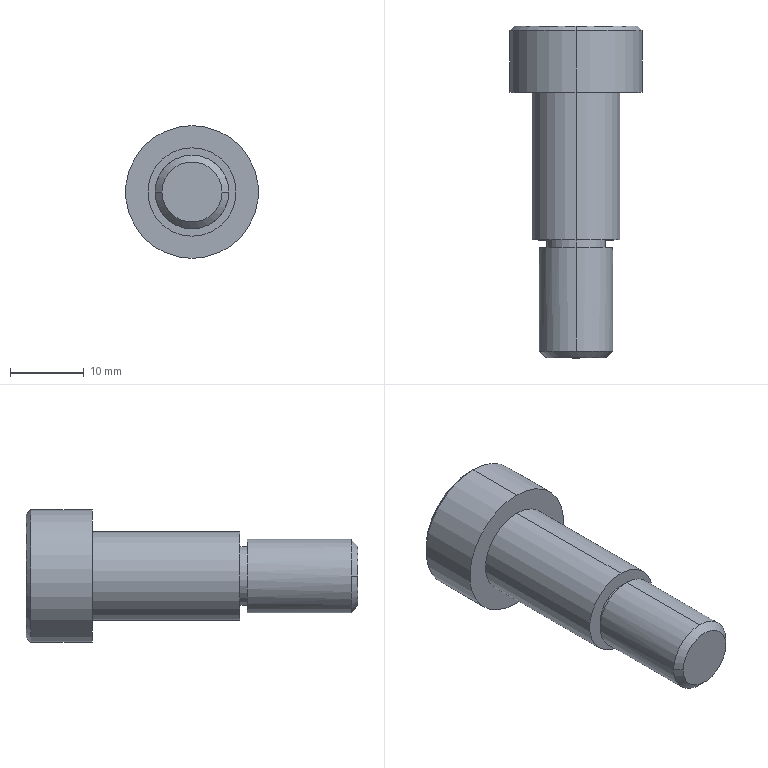Part | SolidWorks | features BaseBody 1, MoveFace 1 | 1 solid | 24 faces | box 18 x 45 x 18 mm | volume 5618 mm3 | plane 12 | cylinder 8 | cone 4 | commonest cylinder face diameters 8 x2 10 x2 12 x2 18 x2
STEP:
#1=CARTESIAN_POINT('',(0.,12.,6.));
#2=VERTEX_POINT('',#1);
#3=CARTESIAN_POINT('',(0.,12.,-6.));
#4=VERTEX_POINT('',#3);
#5=CARTESIAN_POINT('',(0.,12.,0.));
#6=DIRECTION('',(0.,1.,0.));
#7=DIRECTION('',(0.,0.,1.));
#8=AXIS2_PLACEMENT_3D('',#5,#6,#7);
#9=CIRCLE('',#8,6.);
#10=EDGE_CURVE('',#2,#4,#9,.T.);
#11=ORIENTED_EDGE('',*,*,#10,.T.);
#12=CARTESIAN_POINT('',(0.,32.,-6.));
#13=VERTEX_POINT('',#12);
#14=CARTESIAN_POINT('',(0.,0.,-6.));
#15=DIRECTION('',(0.,1.,0.));
#16=VECTOR('',#15,1000.);
#17=LINE('',#14,#16);
#18=EDGE_CURVE('',#4,#13,#17,.T.);
#19=ORIENTED_EDGE('',*,*,#18,.T.);
#20=CARTESIAN_POINT('',(0.,32.,6.));
#21=VERTEX_POINT('',#20);
#22=CARTESIAN_POINT('',(0.,32.,0.));
#23=DIRECTION('',(0.,-1.,0.));
#24=DIRECTION('',(0.,0.,1.));
#25=AXIS2_PLACEMENT_3D('',#22,#23,#24);
#26=CIRCLE('',#25,6.);
#27=EDGE_CURVE('',#13,#21,#26,.T.);
#28=ORIENTED_EDGE('',*,*,#27,.T.);
#29=CARTESIAN_POINT('',(0.,0.,6.));
#30=DIRECTION('',(0.,1.,0.));
#31=VECTOR('',#30,1000.);
#32=LINE('',#29,#31);
#33=EDGE_CURVE('',#2,#21,#32,.T.);
#34=ORIENTED_EDGE('',*,*,#33,.F.);
#35=EDGE_LOOP('',(#11,#19,#28,#34));
#36=FACE_OUTER_BOUND('',#35,.T.);
#37=CARTESIAN_POINT('',(0.,0.,0.));
#38=DIRECTION('',(0.,1.,0.));
#39=DIRECTION('',(0.,0.,1.));
#40=AXIS2_PLACEMENT_3D('',#37,#38,#39);
#41=CYLINDRICAL_SURFACE('',#40,6.);
#42=ADVANCED_FACE('',(#36),#41,.T.);
#43=CARTESIAN_POINT('',(0.,32.,9.));
#44=VERTEX_POINT('',#43);
#45=CARTESIAN_POINT('',(0.,32.,-9.));
#46=VERTEX_POINT('',#45);
#47=CARTESIAN_POINT('',(0.,32.,0.));
#48=DIRECTION('',(0.,1.,0.));
#49=DIRECTION('',(0.,0.,1.));
#50=AXIS2_PLACEMENT_3D('',#47,#48,#49);
#51=CIRCLE('',#50,9.);
#52=EDGE_CURVE('',#44,#46,#51,.T.);
#53=ORIENTED_EDGE('',*,*,#52,.T.);
#54=CARTESIAN_POINT('',(0.,40.4,-9.));
#55=VERTEX_POINT('',#54);
#56=CARTESIAN_POINT('',(0.,0.,-9.));
#57=DIRECTION('',(0.,1.,0.));
#58=VECTOR('',#57,1000.);
#59=LINE('',#56,#58);
#60=EDGE_CURVE('',#46,#55,#59,.T.);
#61=ORIENTED_EDGE('',*,*,#60,.T.);
#62=CARTESIAN_POINT('',(0.,40.4,9.));
#63=VERTEX_POINT('',#62);
#64=CARTESIAN_POINT('',(0.,40.4,0.));
#65=DIRECTION('',(0.,-1.,0.));
#66=DIRECTION('',(0.,0.,1.));
#67=AXIS2_PLACEMENT_3D('',#64,#65,#66);
#68=CIRCLE('',#67,9.);
#69=EDGE_CURVE('',#55,#63,#68,.T.);
#70=ORIENTED_EDGE('',*,*,#69,.T.);
#71=CARTESIAN_POINT('',(0.,0.,9.));
#72=DIRECTION('',(0.,1.,0.));
#73=VECTOR('',#72,1000.);
#74=LINE('',#71,#73);
#75=EDGE_CURVE('',#44,#63,#74,.T.);
#76=ORIENTED_EDGE('',*,*,#75,.F.);
#77=EDGE_LOOP('',(#53,#61,#70,#76));
#78=FACE_OUTER_BOUND('',#77,.T.);
#79=CARTESIAN_POINT('',(0.,0.,0.));
#80=DIRECTION('',(0.,1.,0.));
#81=DIRECTION('',(0.,0.,1.));
#82=AXIS2_PLACEMENT_3D('',#79,#80,#81);
#83=CYLINDRICAL_SURFACE('',#82,9.);
#84=ADVANCED_FACE('',(#78),#83,.T.);
#85=CARTESIAN_POINT('',(0.,11.,4.));
#86=VERTEX_POINT('',#85);
#87=CARTESIAN_POINT('',(0.,11.,-4.));
#88=VERTEX_POINT('',#87);
#89=CARTESIAN_POINT('',(0.,11.,0.));
#90=DIRECTION('',(0.,1.,0.));
#91=DIRECTION('',(0.,0.,1.));
#92=AXIS2_PLACEMENT_3D('',#89,#90,#91);
#93=CIRCLE('',#92,4.);
#94=EDGE_CURVE('',#86,#88,#93,.T.);
#95=ORIENTED_EDGE('',*,*,#94,.T.);
#96=CARTESIAN_POINT('',(0.,12.,-4.));
#97=VERTEX_POINT('',#96);
#98=CARTESIAN_POINT('',(0.,0.,-4.));
#99=DIRECTION('',(0.,1.,0.));
#100=VECTOR('',#99,1000.);
#101=LINE('',#98,#100);
#102=EDGE_CURVE('',#88,#97,#101,.T.);
#103=ORIENTED_EDGE('',*,*,#102,.T.);
#104=CARTESIAN_POINT('',(0.,12.,4.));
#105=VERTEX_POINT('',#104);
#106=CARTESIAN_POINT('',(0.,12.,0.));
#107=DIRECTION('',(0.,-1.,0.));
#108=DIRECTION('',(0.,0.,1.));
#109=AXIS2_PLACEMENT_3D('',#106,#107,#108);
#110=CIRCLE('',#109,4.);
#111=EDGE_CURVE('',#97,#105,#110,.T.);
#112=ORIENTED_EDGE('',*,*,#111,.T.);
#113=CARTESIAN_POINT('',(0.,0.,4.));
#114=DIRECTION('',(0.,1.,0.));
#115=VECTOR('',#114,1000.);
#116=LINE('',#113,#115);
#117=EDGE_CURVE('',#86,#105,#116,.T.);
#118=ORIENTED_EDGE('',*,*,#117,.F.);
#119=EDGE_LOOP('',(#95,#103,#112,#118));
#120=FACE_OUTER_BOUND('',#119,.T.);
#121=CARTESIAN_POINT('',(0.,0.,0.));
#122=DIRECTION('',(0.,1.,0.));
#123=DIRECTION('',(0.,0.,1.));
#124=AXIS2_PLACEMENT_3D('',#121,#122,#123);
#125=CYLINDRICAL_SURFACE('',#124,4.);
#126=ADVANCED_FACE('',(#120),#125,.T.);
#127=CARTESIAN_POINT('',(0.,41.,-8.4));
#128=VERTEX_POINT('',#127);
#129=CARTESIAN_POINT('',(0.,41.,8.4));
#130=VERTEX_POINT('',#129);
#131=CARTESIAN_POINT('',(0.,41.,0.));
#132=DIRECTION('',(0.,-1.,0.));
#133=DIRECTION('',(0.,0.,-1.));
#134=AXIS2_PLACEMENT_3D('',#131,#132,#133);
#135=CIRCLE('',#134,8.4);
#136=EDGE_CURVE('',#128,#130,#135,.T.);
#137=ORIENTED_EDGE('',*,*,#136,.T.);
#138=CARTESIAN_POINT('',(0.,40.4,9.));
#139=DIRECTION('',(0.,-0.7071,0.7071));
#140=VECTOR('',#139,1000.);
#141=LINE('',#138,#140);
#142=EDGE_CURVE('',#130,#63,#141,.T.);
#143=ORIENTED_EDGE('',*,*,#142,.T.);
#144=ORIENTED_EDGE('',*,*,#69,.F.);
#145=CARTESIAN_POINT('',(0.,40.4,-9.));
#146=DIRECTION('',(0.,-0.7071,-0.7071));
#147=VECTOR('',#146,1000.);
#148=LINE('',#145,#147);
#149=EDGE_CURVE('',#128,#55,#148,.T.);
#150=ORIENTED_EDGE('',*,*,#149,.F.);
#151=EDGE_LOOP('',(#137,#143,#144,#150));
#152=FACE_OUTER_BOUND('',#151,.T.);
#153=CARTESIAN_POINT('',(0.,40.4,0.));
#154=DIRECTION('',(0.,-1.,0.));
#155=DIRECTION('',(0.,0.,-1.));
#156=AXIS2_PLACEMENT_3D('',#153,#154,#155);
#157=CONICAL_SURFACE('',#156,9.,0.7854);
#158=ADVANCED_FACE('',(#152),#157,.T.);
#159=CARTESIAN_POINT('',(5.,-3.08,0.));
#160=VERTEX_POINT('',#159);
#161=CARTESIAN_POINT('',(0.,-3.08,-5.));
#162=VERTEX_POINT('',#161);
#163=CARTESIAN_POINT('',(0.,-3.08,0.));
#164=DIRECTION('',(0.,1.,0.));
#165=DIRECTION('',(0.,0.,1.));
#166=AXIS2_PLACEMENT_3D('',#163,#164,#165);
#167=CIRCLE('',#166,5.);
#168=EDGE_CURVE('',#160,#162,#167,.T.);
#169=ORIENTED_EDGE('',*,*,#168,.T.);
#170=CARTESIAN_POINT('',(0.,11.,-5.));
#171=VERTEX_POINT('',#170);
#172=CARTESIAN_POINT('',(0.,0.,-5.));
#173=DIRECTION('',(0.,1.,0.));
#174=VECTOR('',#173,1000.);
#175=LINE('',#172,#174);
#176=EDGE_CURVE('',#162,#171,#175,.T.);
#177=ORIENTED_EDGE('',*,*,#176,.T.);
#178=CARTESIAN_POINT('',(0.,11.,5.));
#179=VERTEX_POINT('',#178);
#180=CARTESIAN_POINT('',(0.,11.,0.));
#181=DIRECTION('',(0.,-1.,0.));
#182=DIRECTION('',(0.,0.,1.));
#183=AXIS2_PLACEMENT_3D('',#180,#181,#182);
#184=CIRCLE('',#183,5.);
#185=EDGE_CURVE('',#171,#179,#184,.T.);
#186=ORIENTED_EDGE('',*,*,#185,.T.);
#187=CARTESIAN_POINT('',(0.,-3.08,5.));
#188=VERTEX_POINT('',#187);
#189=CARTESIAN_POINT('',(0.,0.,5.));
#190=DIRECTION('',(0.,1.,0.));
#191=VECTOR('',#190,1000.);
#192=LINE('',#189,#191);
#193=EDGE_CURVE('',#188,#179,#192,.T.);
#194=ORIENTED_EDGE('',*,*,#193,.F.);
#195=CARTESIAN_POINT('',(0.,-3.08,0.));
#196=DIRECTION('',(0.,1.,0.));
#197=DIRECTION('',(0.,0.,1.));
#198=AXIS2_PLACEMENT_3D('',#195,#196,#197);
#199=CIRCLE('',#198,5.);
#200=EDGE_CURVE('',#188,#160,#199,.T.);
#201=ORIENTED_EDGE('',*,*,#200,.T.);
#202=EDGE_LOOP('',(#169,#177,#186,#194,#201));
#203=FACE_OUTER_BOUND('',#202,.T.);
#204=CARTESIAN_POINT('',(0.,0.,0.));
#205=DIRECTION('',(0.,1.,0.));
#206=DIRECTION('',(0.,0.,1.));
#207=AXIS2_PLACEMENT_3D('',#204,#205,#206);
#208=CYLINDRICAL_SURFACE('',#207,5.);
#209=ADVANCED_FACE('',(#203),#208,.T.);
#210=CARTESIAN_POINT('',(-4.08,-4.,0.));
#211=VERTEX_POINT('',#210);
#212=CARTESIAN_POINT('',(4.08,-4.,0.));
#213=VERTEX_POINT('',#212);
#214=CARTESIAN_POINT('',(0.,-4.,0.));
#215=DIRECTION('',(0.,1.,0.));
#216=DIRECTION('',(-1.,0.,0.));
#217=AXIS2_PLACEMENT_3D('',#214,#215,#216);
#218=CIRCLE('',#217,4.08);
#219=EDGE_CURVE('',#211,#213,#218,.T.);
#220=ORIENTED_EDGE('',*,*,#219,.T.);
#221=CARTESIAN_POINT('',(5.,-3.08,0.));
#222=DIRECTION('',(0.7071,0.7071,0.));
#223=VECTOR('',#222,1000.);
#224=LINE('',#221,#223);
#225=EDGE_CURVE('',#213,#160,#224,.T.);
#226=ORIENTED_EDGE('',*,*,#225,.T.);
#227=ORIENTED_EDGE('',*,*,#200,.F.);
#228=CARTESIAN_POINT('',(-5.,-3.08,0.));
#229=VERTEX_POINT('',#228);
#230=CARTESIAN_POINT('',(0.,-3.08,0.));
#231=DIRECTION('',(0.,1.,0.));
#232=DIRECTION('',(0.,0.,1.));
#233=AXIS2_PLACEMENT_3D('',#230,#231,#232);
#234=CIRCLE('',#233,5.);
#235=EDGE_CURVE('',#229,#188,#234,.T.);
#236=ORIENTED_EDGE('',*,*,#235,.F.);
#237=CARTESIAN_POINT('',(-5.,-3.08,0.));
#238=DIRECTION('',(-0.7071,0.7071,0.));
#239=VECTOR('',#238,1000.);
#240=LINE('',#237,#239);
#241=EDGE_CURVE('',#211,#229,#240,.T.);
#242=ORIENTED_EDGE('',*,*,#241,.F.);
#243=EDGE_LOOP('',(#220,#226,#227,#236,#242));
#244=FACE_OUTER_BOUND('',#243,.T.);
#245=CARTESIAN_POINT('',(0.,-3.08,0.));
#246=DIRECTION('',(0.,1.,0.));
#247=DIRECTION('',(-1.,0.,0.));
#248=AXIS2_PLACEMENT_3D('',#245,#246,#247);
#249=CONICAL_SURFACE('',#248,5.,0.7854);
#250=ADVANCED_FACE('',(#244),#249,.T.);
#251=ORIENTED_EDGE('',*,*,#18,.F.);
#252=CARTESIAN_POINT('',(0.,12.,0.));
#253=DIRECTION('',(0.,1.,0.));
#254=DIRECTION('',(0.,0.,1.));
#255=AXIS2_PLACEMENT_3D('',#252,#253,#254);
#256=CIRCLE('',#255,6.);
#257=EDGE_CURVE('',#4,#2,#256,.T.);
#258=ORIENTED_EDGE('',*,*,#257,.T.);
#259=ORIENTED_EDGE('',*,*,#33,.T.);
#260=CARTESIAN_POINT('',(0.,32.,0.));
#261=DIRECTION('',(0.,-1.,0.));
#262=DIRECTION('',(0.,0.,1.));
#263=AXIS2_PLACEMENT_3D('',#260,#261,#262);
#264=CIRCLE('',#263,6.);
#265=EDGE_CURVE('',#21,#13,#264,.T.);
#266=ORIENTED_EDGE('',*,*,#265,.T.);
#267=EDGE_LOOP('',(#251,#258,#259,#266));
#268=FACE_OUTER_BOUND('',#267,.T.);
#269=CARTESIAN_POINT('',(0.,0.,0.));
#270=DIRECTION('',(0.,1.,0.));
#271=DIRECTION('',(0.,0.,1.));
#272=AXIS2_PLACEMENT_3D('',#269,#270,#271);
#273=CYLINDRICAL_SURFACE('',#272,6.);
#274=ADVANCED_FACE('',(#268),#273,.T.);
#275=ORIENTED_EDGE('',*,*,#52,.F.);
#276=CARTESIAN_POINT('',(0.,32.,0.));
#277=DIRECTION('',(0.,1.,0.));
#278=DIRECTION('',(0.,0.,1.));
#279=AXIS2_PLACEMENT_3D('',#276,#277,#278);
#280=CIRCLE('',#279,9.);
#281=EDGE_CURVE('',#46,#44,#280,.T.);
#282=ORIENTED_EDGE('',*,*,#281,.F.);
#283=EDGE_LOOP('',(#275,#282));
#284=FACE_OUTER_BOUND('',#283,.T.);
#285=ORIENTED_EDGE('',*,*,#265,.F.);
#286=ORIENTED_EDGE('',*,*,#27,.F.);
#287=EDGE_LOOP('',(#285,#286));
#288=FACE_BOUND('',#287,.T.);
#289=CARTESIAN_POINT('',(9.,32.,0.));
#290=DIRECTION('',(0.,1.,0.));
#291=DIRECTION('',(0.,0.,1.));
#292=AXIS2_PLACEMENT_3D('',#289,#290,#291);
#293=PLANE('',#292);
#294=ADVANCED_FACE('',(#284,#288),#293,.F.);
#295=ORIENTED_EDGE('',*,*,#10,.F.);
#296=ORIENTED_EDGE('',*,*,#257,.F.);
#297=EDGE_LOOP('',(#295,#296));
#298=FACE_OUTER_BOUND('',#297,.T.);
#299=CARTESIAN_POINT('',(0.,12.,0.));
#300=DIRECTION('',(0.,-1.,0.));
#301=DIRECTION('',(0.,0.,1.));
#302=AXIS2_PLACEMENT_3D('',#299,#300,#301);
#303=CIRCLE('',#302,4.);
#304=EDGE_CURVE('',#105,#97,#303,.T.);
#305=ORIENTED_EDGE('',*,*,#304,.F.);
#306=ORIENTED_EDGE('',*,*,#111,.F.);
#307=EDGE_LOOP('',(#305,#306));
#308=FACE_BOUND('',#307,.T.);
#309=CARTESIAN_POINT('',(6.,12.,0.));
#310=DIRECTION('',(0.,1.,0.));
#311=DIRECTION('',(0.,0.,1.));
#312=AXIS2_PLACEMENT_3D('',#309,#310,#311);
#313=PLANE('',#312);
#314=ADVANCED_FACE('',(#298,#308),#313,.F.);
#315=ORIENTED_EDGE('',*,*,#60,.F.);
#316=ORIENTED_EDGE('',*,*,#281,.T.);
#317=ORIENTED_EDGE('',*,*,#75,.T.);
#318=CARTESIAN_POINT('',(0.,40.4,0.));
#319=DIRECTION('',(0.,-1.,0.));
#320=DIRECTION('',(0.,0.,1.));
#321=AXIS2_PLACEMENT_3D('',#318,#319,#320);
#322=CIRCLE('',#321,9.);
#323=EDGE_CURVE('',#63,#55,#322,.T.);
#324=ORIENTED_EDGE('',*,*,#323,.T.);
#325=EDGE_LOOP('',(#315,#316,#317,#324));
#326=FACE_OUTER_BOUND('',#325,.T.);
#327=CARTESIAN_POINT('',(0.,0.,0.));
#328=DIRECTION('',(0.,1.,0.));
#329=DIRECTION('',(0.,0.,1.));
#330=AXIS2_PLACEMENT_3D('',#327,#328,#329);
#331=CYLINDRICAL_SURFACE('',#330,9.);
#332=ADVANCED_FACE('',(#326),#331,.T.);
#333=ORIENTED_EDGE('',*,*,#102,.F.);
#334=CARTESIAN_POINT('',(0.,11.,0.));
#335=DIRECTION('',(0.,1.,0.));
#336=DIRECTION('',(0.,0.,1.));
#337=AXIS2_PLACEMENT_3D('',#334,#335,#336);
#338=CIRCLE('',#337,4.);
#339=EDGE_CURVE('',#88,#86,#338,.T.);
#340=ORIENTED_EDGE('',*,*,#339,.T.);
#341=ORIENTED_EDGE('',*,*,#117,.T.);
#342=ORIENTED_EDGE('',*,*,#304,.T.);
#343=EDGE_LOOP('',(#333,#340,#341,#342));
#344=FACE_OUTER_BOUND('',#343,.T.);
#345=CARTESIAN_POINT('',(0.,0.,0.));
#346=DIRECTION('',(0.,1.,0.));
#347=DIRECTION('',(0.,0.,1.));
#348=AXIS2_PLACEMENT_3D('',#345,#346,#347);
#349=CYLINDRICAL_SURFACE('',#348,4.);
#350=ADVANCED_FACE('',(#344),#349,.T.);
#351=ORIENTED_EDGE('',*,*,#142,.F.);
#352=CARTESIAN_POINT('',(0.,41.,0.));
#353=DIRECTION('',(0.,-1.,0.));
#354=DIRECTION('',(0.,0.,-1.));
#355=AXIS2_PLACEMENT_3D('',#352,#353,#354);
#356=CIRCLE('',#355,8.4);
#357=EDGE_CURVE('',#130,#128,#356,.T.);
#358=ORIENTED_EDGE('',*,*,#357,.T.);
#359=ORIENTED_EDGE('',*,*,#149,.T.);
#360=ORIENTED_EDGE('',*,*,#323,.F.);
#361=EDGE_LOOP('',(#351,#358,#359,#360));
#362=FACE_OUTER_BOUND('',#361,.T.);
#363=CARTESIAN_POINT('',(0.,40.4,0.));
#364=DIRECTION('',(0.,-1.,0.));
#365=DIRECTION('',(0.,0.,-1.));
#366=AXIS2_PLACEMENT_3D('',#363,#364,#365);
#367=CONICAL_SURFACE('',#366,9.,0.7854);
#368=ADVANCED_FACE('',(#362),#367,.T.);
#369=ORIENTED_EDGE('',*,*,#94,.F.);
#370=ORIENTED_EDGE('',*,*,#339,.F.);
#371=EDGE_LOOP('',(#369,#370));
#372=FACE_BOUND('',#371,.T.);
#373=CARTESIAN_POINT('',(0.,11.,0.));
#374=DIRECTION('',(0.,-1.,0.));
#375=DIRECTION('',(0.,0.,1.));
#376=AXIS2_PLACEMENT_3D('',#373,#374,#375);
#377=CIRCLE('',#376,5.);
#378=EDGE_CURVE('',#179,#171,#377,.T.);
#379=ORIENTED_EDGE('',*,*,#378,.F.);
#380=ORIENTED_EDGE('',*,*,#185,.F.);
#381=EDGE_LOOP('',(#379,#380));
#382=FACE_OUTER_BOUND('',#381,.T.);
#383=CARTESIAN_POINT('',(4.,11.,0.));
#384=DIRECTION('',(0.,-1.,0.));
#385=DIRECTION('',(0.,0.,-1.));
#386=AXIS2_PLACEMENT_3D('',#383,#384,#385);
#387=PLANE('',#386);
#388=ADVANCED_FACE('',(#372,#382),#387,.F.);
#389=CARTESIAN_POINT('',(-3.,41.,1.732));
#390=VERTEX_POINT('',#389);
#391=CARTESIAN_POINT('',(0.,41.,3.464));
#392=VERTEX_POINT('',#391);
#393=CARTESIAN_POINT('',(-3.,41.,1.732));
#394=DIRECTION('',(0.866,0.,0.5));
#395=VECTOR('',#394,1000.);
#396=LINE('',#393,#395);
#397=EDGE_CURVE('',#390,#392,#396,.T.);
#398=ORIENTED_EDGE('',*,*,#397,.F.);
#399=CARTESIAN_POINT('',(-3.,41.,-1.732));
#400=VERTEX_POINT('',#399);
#401=CARTESIAN_POINT('',(-3.,41.,0.));
#402=DIRECTION('',(0.,0.,1.));
#403=VECTOR('',#402,1000.);
#404=LINE('',#401,#403);
#405=EDGE_CURVE('',#400,#390,#404,.T.);
#406=ORIENTED_EDGE('',*,*,#405,.F.);
#407=CARTESIAN_POINT('',(0.,41.,-3.464));
#408=VERTEX_POINT('',#407);
#409=CARTESIAN_POINT('',(0.,41.,-3.464));
#410=DIRECTION('',(-0.866,0.,0.5));
#411=VECTOR('',#410,1000.);
#412=LINE('',#409,#411);
#413=EDGE_CURVE('',#408,#400,#412,.T.);
#414=ORIENTED_EDGE('',*,*,#413,.F.);
#415=CARTESIAN_POINT('',(3.,41.,-1.732));
#416=VERTEX_POINT('',#415);
#417=CARTESIAN_POINT('',(3.,41.,-1.732));
#418=DIRECTION('',(-0.866,0.,-0.5));
#419=VECTOR('',#418,1000.);
#420=LINE('',#417,#419);
#421=EDGE_CURVE('',#416,#408,#420,.T.);
#422=ORIENTED_EDGE('',*,*,#421,.F.);
#423=CARTESIAN_POINT('',(3.,41.,1.732));
#424=VERTEX_POINT('',#423);
#425=CARTESIAN_POINT('',(3.,41.,0.));
#426=DIRECTION('',(0.,0.,-1.));
#427=VECTOR('',#426,1000.);
#428=LINE('',#425,#427);
#429=EDGE_CURVE('',#424,#416,#428,.T.);
#430=ORIENTED_EDGE('',*,*,#429,.F.);
#431=CARTESIAN_POINT('',(0.,41.,3.464));
#432=DIRECTION('',(0.866,0.,-0.5));
#433=VECTOR('',#432,1000.);
#434=LINE('',#431,#433);
#435=EDGE_CURVE('',#392,#424,#434,.T.);
#436=ORIENTED_EDGE('',*,*,#435,.F.);
#437=EDGE_LOOP('',(#398,#406,#414,#422,#430,#436));
#438=FACE_BOUND('',#437,.T.);
#439=ORIENTED_EDGE('',*,*,#136,.F.);
#440=ORIENTED_EDGE('',*,*,#357,.F.);
#441=EDGE_LOOP('',(#439,#440));
#442=FACE_OUTER_BOUND('',#441,.T.);
#443=CARTESIAN_POINT('',(0.,41.,0.));
#444=DIRECTION('',(0.,-1.,0.));
#445=DIRECTION('',(0.,0.,-1.));
#446=AXIS2_PLACEMENT_3D('',#443,#444,#445);
#447=PLANE('',#446);
#448=ADVANCED_FACE('',(#438,#442),#447,.F.);
#449=ORIENTED_EDGE('',*,*,#176,.F.);
#450=CARTESIAN_POINT('',(0.,-3.08,0.));
#451=DIRECTION('',(0.,1.,0.));
#452=DIRECTION('',(0.,0.,1.));
#453=AXIS2_PLACEMENT_3D('',#450,#451,#452);
#454=CIRCLE('',#453,5.);
#455=EDGE_CURVE('',#162,#229,#454,.T.);
#456=ORIENTED_EDGE('',*,*,#455,.T.);
#457=ORIENTED_EDGE('',*,*,#235,.T.);
#458=ORIENTED_EDGE('',*,*,#193,.T.);
#459=ORIENTED_EDGE('',*,*,#378,.T.);
#460=EDGE_LOOP('',(#449,#456,#457,#458,#459));
#461=FACE_OUTER_BOUND('',#460,.T.);
#462=CARTESIAN_POINT('',(0.,0.,0.));
#463=DIRECTION('',(0.,1.,0.));
#464=DIRECTION('',(0.,0.,1.));
#465=AXIS2_PLACEMENT_3D('',#462,#463,#464);
#466=CYLINDRICAL_SURFACE('',#465,5.);
#467=ADVANCED_FACE('',(#461),#466,.T.);
#468=CARTESIAN_POINT('',(3.,36.5,1.732));
#469=VERTEX_POINT('',#468);
#470=CARTESIAN_POINT('',(3.,36.5,1.732));
#471=DIRECTION('',(0.,1.,0.));
#472=VECTOR('',#471,1000.);
#473=LINE('',#470,#472);
#474=EDGE_CURVE('',#469,#424,#473,.T.);
#475=ORIENTED_EDGE('',*,*,#474,.F.);
#476=CARTESIAN_POINT('',(0.,36.5,3.464));
#477=VERTEX_POINT('',#476);
#478=CARTESIAN_POINT('',(0.,36.5,3.464));
#479=DIRECTION('',(0.866,0.,-0.5));
#480=VECTOR('',#479,1000.);
#481=LINE('',#478,#480);
#482=EDGE_CURVE('',#477,#469,#481,.T.);
#483=ORIENTED_EDGE('',*,*,#482,.F.);
#484=CARTESIAN_POINT('',(0.,36.5,3.464));
#485=DIRECTION('',(0.,-1.,0.));
#486=VECTOR('',#485,1000.);
#487=LINE('',#484,#486);
#488=EDGE_CURVE('',#392,#477,#487,.T.);
#489=ORIENTED_EDGE('',*,*,#488,.F.);
#490=ORIENTED_EDGE('',*,*,#435,.T.);
#491=EDGE_LOOP('',(#475,#483,#489,#490));
#492=FACE_OUTER_BOUND('',#491,.T.);
#493=CARTESIAN_POINT('',(0.,36.5,3.464));
#494=DIRECTION('',(0.5,0.,0.866));
#495=DIRECTION('',(0.866,0.,-0.5));
#496=AXIS2_PLACEMENT_3D('',#493,#494,#495);
#497=PLANE('',#496);
#498=ADVANCED_FACE('',(#492),#497,.F.);
#499=ORIENTED_EDGE('',*,*,#488,.T.);
#500=CARTESIAN_POINT('',(-3.,36.5,1.732));
#501=VERTEX_POINT('',#500);
#502=CARTESIAN_POINT('',(-3.,36.5,1.732));
#503=DIRECTION('',(0.866,0.,0.5));
#504=VECTOR('',#503,1000.);
#505=LINE('',#502,#504);
#506=EDGE_CURVE('',#501,#477,#505,.T.);
#507=ORIENTED_EDGE('',*,*,#506,.F.);
#508=CARTESIAN_POINT('',(-3.,36.5,1.732));
#509=DIRECTION('',(0.,-1.,0.));
#510=VECTOR('',#509,1000.);
#511=LINE('',#508,#510);
#512=EDGE_CURVE('',#390,#501,#511,.T.);
#513=ORIENTED_EDGE('',*,*,#512,.F.);
#514=ORIENTED_EDGE('',*,*,#397,.T.);
#515=EDGE_LOOP('',(#499,#507,#513,#514));
#516=FACE_OUTER_BOUND('',#515,.T.);
#517=CARTESIAN_POINT('',(-3.,36.5,1.732));
#518=DIRECTION('',(-0.5,0.,0.866));
#519=DIRECTION('',(0.866,0.,0.5));
#520=AXIS2_PLACEMENT_3D('',#517,#518,#519);
#521=PLANE('',#520);
#522=ADVANCED_FACE('',(#516),#521,.F.);
#523=ORIENTED_EDGE('',*,*,#512,.T.);
#524=CARTESIAN_POINT('',(-3.,36.5,-1.732));
#525=VERTEX_POINT('',#524);
#526=CARTESIAN_POINT('',(-3.,36.5,-1.732));
#527=DIRECTION('',(0.,0.,1.));
#528=VECTOR('',#527,1000.);
#529=LINE('',#526,#528);
#530=EDGE_CURVE('',#525,#501,#529,.T.);
#531=ORIENTED_EDGE('',*,*,#530,.F.);
#532=CARTESIAN_POINT('',(-3.,36.5,-1.732));
#533=DIRECTION('',(0.,-1.,0.));
#534=VECTOR('',#533,1000.);
#535=LINE('',#532,#534);
#536=EDGE_CURVE('',#400,#525,#535,.T.);
#537=ORIENTED_EDGE('',*,*,#536,.F.);
#538=ORIENTED_EDGE('',*,*,#405,.T.);
#539=EDGE_LOOP('',(#523,#531,#537,#538));
#540=FACE_OUTER_BOUND('',#539,.T.);
#541=CARTESIAN_POINT('',(-3.,36.5,-1.732));
#542=DIRECTION('',(-1.,0.,0.));
#543=DIRECTION('',(0.,0.,1.));
#544=AXIS2_PLACEMENT_3D('',#541,#542,#543);
#545=PLANE('',#544);
#546=ADVANCED_FACE('',(#540),#545,.F.);
#547=ORIENTED_EDGE('',*,*,#536,.T.);
#548=CARTESIAN_POINT('',(0.,36.5,-3.464));
#549=VERTEX_POINT('',#548);
#550=CARTESIAN_POINT('',(0.,36.5,-3.464));
#551=DIRECTION('',(-0.866,0.,0.5));
#552=VECTOR('',#551,1000.);
#553=LINE('',#550,#552);
#554=EDGE_CURVE('',#549,#525,#553,.T.);
#555=ORIENTED_EDGE('',*,*,#554,.F.);
#556=CARTESIAN_POINT('',(0.,36.5,-3.464));
#557=DIRECTION('',(0.,-1.,0.));
#558=VECTOR('',#557,1000.);
#559=LINE('',#556,#558);
#560=EDGE_CURVE('',#408,#549,#559,.T.);
#561=ORIENTED_EDGE('',*,*,#560,.F.);
#562=ORIENTED_EDGE('',*,*,#413,.T.);
#563=EDGE_LOOP('',(#547,#555,#561,#562));
#564=FACE_OUTER_BOUND('',#563,.T.);
#565=CARTESIAN_POINT('',(0.,36.5,-3.464));
#566=DIRECTION('',(-0.5,0.,-0.866));
#567=DIRECTION('',(-0.866,0.,0.5));
#568=AXIS2_PLACEMENT_3D('',#565,#566,#567);
#569=PLANE('',#568);
#570=ADVANCED_FACE('',(#564),#569,.F.);
#571=ORIENTED_EDGE('',*,*,#560,.T.);
#572=CARTESIAN_POINT('',(3.,36.5,-1.732));
#573=VERTEX_POINT('',#572);
#574=CARTESIAN_POINT('',(3.,36.5,-1.732));
#575=DIRECTION('',(-0.866,0.,-0.5));
#576=VECTOR('',#575,1000.);
#577=LINE('',#574,#576);
#578=EDGE_CURVE('',#573,#549,#577,.T.);
#579=ORIENTED_EDGE('',*,*,#578,.F.);
#580=CARTESIAN_POINT('',(3.,36.5,-1.732));
#581=DIRECTION('',(0.,-1.,0.));
#582=VECTOR('',#581,1000.);
#583=LINE('',#580,#582);
#584=EDGE_CURVE('',#416,#573,#583,.T.);
#585=ORIENTED_EDGE('',*,*,#584,.F.);
#586=ORIENTED_EDGE('',*,*,#421,.T.);
#587=EDGE_LOOP('',(#571,#579,#585,#586));
#588=FACE_OUTER_BOUND('',#587,.T.);
#589=CARTESIAN_POINT('',(3.,36.5,-1.732));
#590=DIRECTION('',(0.5,0.,-0.866));
#591=DIRECTION('',(-0.866,0.,-0.5));
#592=AXIS2_PLACEMENT_3D('',#589,#590,#591);
#593=PLANE('',#592);
#594=ADVANCED_FACE('',(#588),#593,.F.);
#595=ORIENTED_EDGE('',*,*,#429,.T.);
#596=ORIENTED_EDGE('',*,*,#584,.T.);
#597=CARTESIAN_POINT('',(3.,36.5,1.732));
#598=DIRECTION('',(0.,0.,-1.));
#599=VECTOR('',#598,1000.);
#600=LINE('',#597,#599);
#601=EDGE_CURVE('',#469,#573,#600,.T.);
#602=ORIENTED_EDGE('',*,*,#601,.F.);
#603=ORIENTED_EDGE('',*,*,#474,.T.);
#604=EDGE_LOOP('',(#595,#596,#602,#603));
#605=FACE_OUTER_BOUND('',#604,.T.);
#606=CARTESIAN_POINT('',(3.,36.5,1.732));
#607=DIRECTION('',(1.,0.,0.));
#608=DIRECTION('',(0.,0.,-1.));
#609=AXIS2_PLACEMENT_3D('',#606,#607,#608);
#610=PLANE('',#609);
#611=ADVANCED_FACE('',(#605),#610,.F.);
#612=ORIENTED_EDGE('',*,*,#225,.F.);
#613=CARTESIAN_POINT('',(0.,-4.,0.));
#614=DIRECTION('',(0.,1.,0.));
#615=DIRECTION('',(-1.,0.,0.));
#616=AXIS2_PLACEMENT_3D('',#613,#614,#615);
#617=CIRCLE('',#616,4.08);
#618=EDGE_CURVE('',#213,#211,#617,.T.);
#619=ORIENTED_EDGE('',*,*,#618,.T.);
#620=ORIENTED_EDGE('',*,*,#241,.T.);
#621=ORIENTED_EDGE('',*,*,#455,.F.);
#622=ORIENTED_EDGE('',*,*,#168,.F.);
#623=EDGE_LOOP('',(#612,#619,#620,#621,#622));
#624=FACE_OUTER_BOUND('',#623,.T.);
#625=CARTESIAN_POINT('',(0.,-3.08,0.));
#626=DIRECTION('',(0.,1.,0.));
#627=DIRECTION('',(-1.,0.,0.));
#628=AXIS2_PLACEMENT_3D('',#625,#626,#627);
#629=CONICAL_SURFACE('',#628,5.,0.7854);
#630=ADVANCED_FACE('',(#624),#629,.T.);
#631=ORIENTED_EDGE('',*,*,#578,.T.);
#632=ORIENTED_EDGE('',*,*,#554,.T.);
#633=ORIENTED_EDGE('',*,*,#530,.T.);
#634=ORIENTED_EDGE('',*,*,#506,.T.);
#635=ORIENTED_EDGE('',*,*,#482,.T.);
#636=ORIENTED_EDGE('',*,*,#601,.T.);
#637=EDGE_LOOP('',(#631,#632,#633,#634,#635,#636));
#638=FACE_OUTER_BOUND('',#637,.T.);
#639=CARTESIAN_POINT('',(0.,36.5,0.));
#640=DIRECTION('',(0.,1.,0.));
#641=DIRECTION('',(0.,0.,1.));
#642=AXIS2_PLACEMENT_3D('',#639,#640,#641);
#643=PLANE('',#642);
#644=ADVANCED_FACE('',(#638),#643,.T.);
#645=ORIENTED_EDGE('',*,*,#219,.F.);
#646=ORIENTED_EDGE('',*,*,#618,.F.);
#647=EDGE_LOOP('',(#645,#646));
#648=FACE_OUTER_BOUND('',#647,.T.);
#649=CARTESIAN_POINT('',(4.08,-4.,0.));
#650=DIRECTION('',(0.,1.,0.));
#651=DIRECTION('',(0.,0.,1.));
#652=AXIS2_PLACEMENT_3D('',#649,#650,#651);
#653=PLANE('',#652);
#654=ADVANCED_FACE('',(#648),#653,.F.);
#655=CLOSED_SHELL('',(#42,#84,#126,#158,#209,#250,#274,#294,#314,#332,#350,#368,#388,#448,#467,#498,#522,#546,#570,#594,#611,#630,#644,#654));
#656=MANIFOLD_SOLID_BREP('',#655);
#657=CARTESIAN_POINT('',(0.,0.,0.));
#658=DIRECTION('',(0.,0.,1.));
#659=DIRECTION('',(1.,0.,0.));
#660=AXIS2_PLACEMENT_3D('',#657,#658,#659);
#661=(LENGTH_UNIT()NAMED_UNIT(*)SI_UNIT(.MILLI.,.METRE.));
#662=UNCERTAINTY_MEASURE_WITH_UNIT(LENGTH_MEASURE(0.00001),#661,'','');
#663=(NAMED_UNIT(*)PLANE_ANGLE_UNIT()SI_UNIT($,.RADIAN.));
#664=(NAMED_UNIT(*)SI_UNIT($,.STERADIAN.)SOLID_ANGLE_UNIT());
#665=(GEOMETRIC_REPRESENTATION_CONTEXT(3)GLOBAL_UNCERTAINTY_ASSIGNED_CONTEXT((#662))GLOBAL_UNIT_ASSIGNED_CONTEXT((#661,#663,#664))REPRESENTATION_CONTEXT('',''));
#666=ADVANCED_BREP_SHAPE_REPRESENTATION('',(#656,#660),#665);